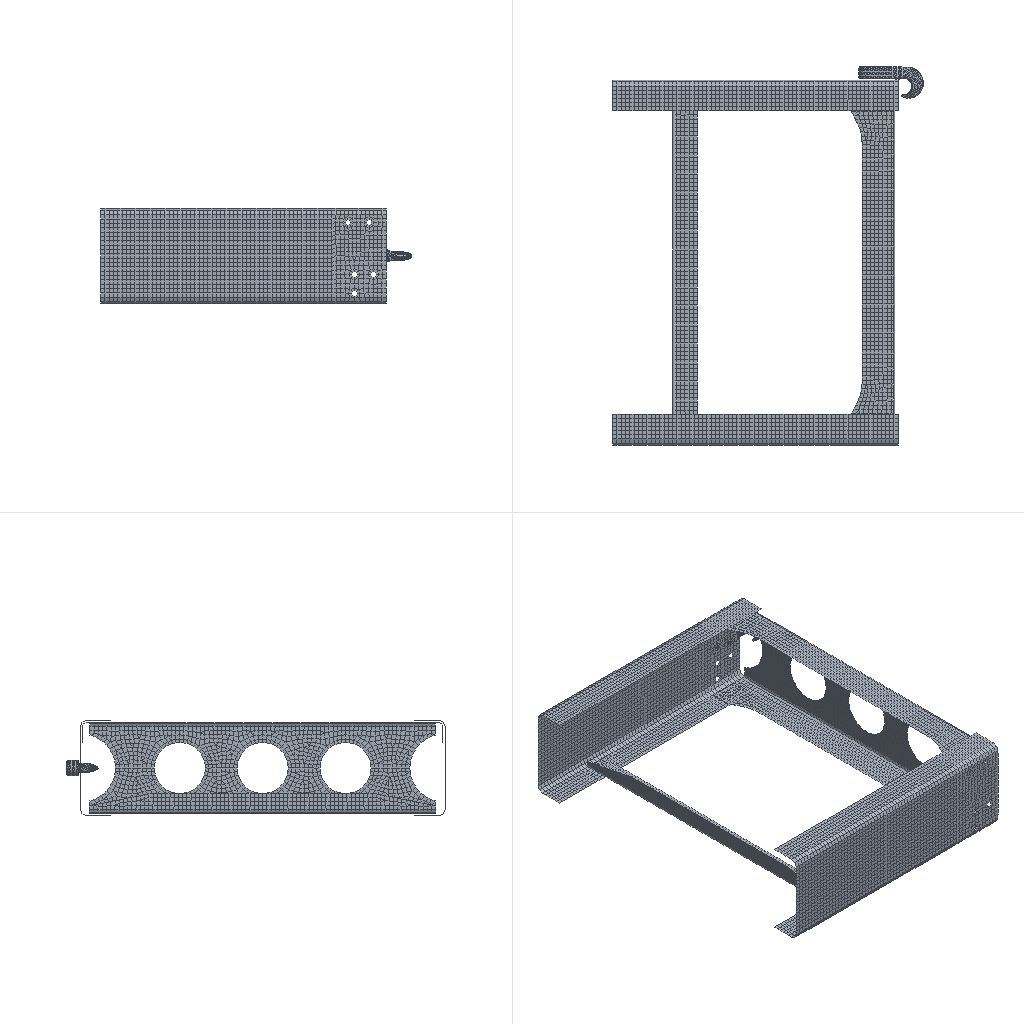Simulation study | nastran
Set-up summary:
category,name,step,type,value,unit,region
solver,nx_nastran
units,not stated in the deck,,not stated
analysis,deck,,static,static
analysis,solution,,SOL,101
load_step,SUBCASE 1,1,SUBCASE,SPC=1 LOAD=2
load_step,SUBCASE 2,2,SUBCASE,SPC=1 LOAD=3
load_step,SUBCASE 3,3,SUBCASE,SPC=1 LOAD=4
load_step,requested,,,3
mesh,nodes,,,35361
mesh,elements,,,24231
element_type,CQUAD4,,shell,8299
element_type,CTETRA,,solid,15807
element_type,CTRIA3,,shell,125
load,load commands in deck,,count,3
bc,support commands in deck,,count,71
check,setup vs results,,match,"every grid point's frame and coordinates and every element id; grid points of CQUAD4, CTETRA, CTRIA3 elements"
Nastran input file, long lists of numbers shortened:
$$------------------------------------------------------------------------------$
$$                                                                              $
$$ NASTRAN Input Deck Generated by HyperMesh Version  : 9.0b121                 $
$$ Generated using HyperMesh-Nastran Template Version : 9.0b121
$$                                                                              $
$$   Template:  general                                                         $
$$                                                                              $
$$------------------------------------------------------------------------------$
$$------------------------------------------------------------------------------$
$$                      Executive Control Cards                                 $
$$------------------------------------------------------------------------------$
SOL 101
CEND
$$------------------------------------------------------------------------------$
$$                      Case Control Cards                                      $
$$------------------------------------------------------------------------------$
  DISPLACEMENT(PLOT) = ALL
  STRESS(PLOT) = ALL
  STRAIN(PLOT) = ALL
$
$HMNAME LOADSTEP               1"Step_Fr"
SUBCASE       1
  LABEL=     Step_Fr
  SPC =        1
  LOAD =        2
$
$HMNAME LOADSTEP               2"Step_Rr"
SUBCASE       2
  LABEL=     Step_Rr
  SPC =        1
  LOAD =        3
$
$HMNAME LOADSTEP               3"Step_Fr30"
SUBCASE       3
  LABEL=     Step_Fr30
  SPC =        1
  LOAD =        4
$$------------------------------------------------------------------------------$
$$                      Bulk Data Cards                                         $
$$------------------------------------------------------------------------------$
BEGIN BULK
PARAM,BAILOUT,-1
PARAM,POST,-1
$$
$$  GRID Data
$$
GRID          41        7505.0  429.5   -36.1424
GRID          42        7495.678429.5   -36.1424
$ (35359 more lines like these left out)
$$
$$  SPOINT Data
$$
$$
$$------------------------------------------------------------------------------$
$$             Group Definitions                                                $
$$------------------------------------------------------------------------------$
$$
$$ RBE2 Elements - Multiple dependent nodes
$$
RBE2      816977  208944  123456   47054   47061   47063   47089   47093+
+          47103   47104   47105   47118   47313   47314   47317   47319+
+          47572   47573   47955   95763   95764   95765   95766   95767+
+          95768   95769   95770  100084  100085  100086  100087  100088+
+         100089  100090  100091
RBE2      816978  208945  123456   47055   47086   47088   47092   47094+
+          47095   47096   47097   47098   47099   47100   47101   47102+
+          47116   47117   47518  198488  198489  198490  198491  198492+
+         198493  198494  198495  202808  202809  202810  202811  202812+
+         202813  202814  202815
$ (203 more lines like these left out)
$
$HMMOVE  2801018
$         816977THRU      816978  836465  836464  836534  836533  836461  836460
$         836463  836462  836535THRU      836536  830313
$
$$
$$  CTRIA3 Data
$$
CTRIA3     47154       9   47518   47117   47517
CTRIA3     47155       9   47518   47519   47055
$ (123 more lines like these left out)
$
$HMMOVE  2801011
$          47154THRU       47155   47158THRU       47159   47161   47173   47186
$          47318   47320THRU       47321   47324THRU       47325   47613   47626
$
$
$HMMOVE  2801012
$         834877  834870  834130  834123  834118  834115  834091  834090  834077
$         834076  834074  834062  834043  834030  834012  834010  833981  833950
$         833948  833942  833941  833918  833911  833906  833903  833896  834234
$         834239  834254  834259  833854  834747  834220  834216  834213  834204
$         834192  834188  834173  834169  834163  834151  833845  833815  833809
$         833805  833800  833789  833770  833747  833741  833733  833730  834652
$         834626  834796  834882  834929  834953THRU      834954  834967THRU
$         834968  834970  834982  835001  835014  835032  835034  835063  835094
$         835096  835102THRU      835103  835126  835133  835138  835141  835148
$         835164  835169  835184  835189  835231  835307  835445  835449  835452
$         835461  835473  835477  835492  835496  835502  835514  835526  835556
$         835562  835566  835571  835582  835601  835873  835879  835887  835890
$         836029  836203  836235
$
$
$HMMOVE  2801014
$             25  830596  836530
$
$
$  CQUAD4 Elements
$
CQUAD4     47132       9   47088   47086   47099   47101
CQUAD4     47133       9   47096   47088   47101   47100
$ (8297 more lines like these left out)
$
$HMMOVE  2801011
$          47132THRU       47153   47156THRU       47157   47160   47162THRU
$          47172   47174THRU       47185   47187THRU       47317   47319   47322
$ (311 more lines like these left out)
CTETRA     20709      13   13379   12090   12470   12640   27410   20414+
+          27170   27329   24252   28082
CTETRA     20710      13   12059   12400   13340   13132   14523   27188+
+          28002   24986   25798   27422
$ (31610 more lines like these left out)
$
$HMMOVE  2801017
$          20709THRU       21708   19709THRU       20708   18709THRU       19708
$          17709THRU       18708   16709THRU       17708   15709THRU       16708
$ (42 more lines like these left out)
PSHELL         9      355.0           35              35
$
$HMNAME PROP                  12"Sheel_600T" 4
$HWCOLOR PROP                 12       3
PSHELL        12      356.0           35              35
$$
$$  PSOLID Data
$
$HMNAME PROP                  13"Solid" 5
$HWCOLOR PROP                 13       3
PSOLID        13      35
$$
$$------------------------------------------------------------------------------$
$$                      Material Definition Cards                               $
$$------------------------------------------------------------------------------$
$$--------------------------------------------------------------
$$ HYPERMESH TAGS
$$--------------------------------------------------------------
$$BEGIN TAGS
$$END TAGS
$$
$$  MAT1 Data
$
$HMNAME MAT                   35"Steel" "MAT1"
$HWCOLOR MAT                  35       6
MAT1          35210000.0        0.3     7.80E-09
$$
$$
$$
$$------------------------------------------------------------------------------$
$ (43 more lines like these left out)
SPC            1  202238  1234560.0
SPC            1  201975  1234560.0
SPC            1  201976  1234560.0
SPC            1  201970  1234560.0
$ (67 more lines like these left out)
$$
$$  FORCE Data
$$
FORCE          4  220970       01.0     50964.730.0     -29424.5
FORCE          3  220970       01.0     58849.0 0.0     0.0
FORCE          2  220970       01.0     -58849.00.0     0.0
$HMASSEM   28011       3 2801
$HMASSEM_IDS     2801011 2801012 2801014
$
ENDDATA
Results summary:
result,analysis,,,static
result,last_loadstep,,,3
result,primary field,,,displacements
result,max displacement,,,3.865,model units